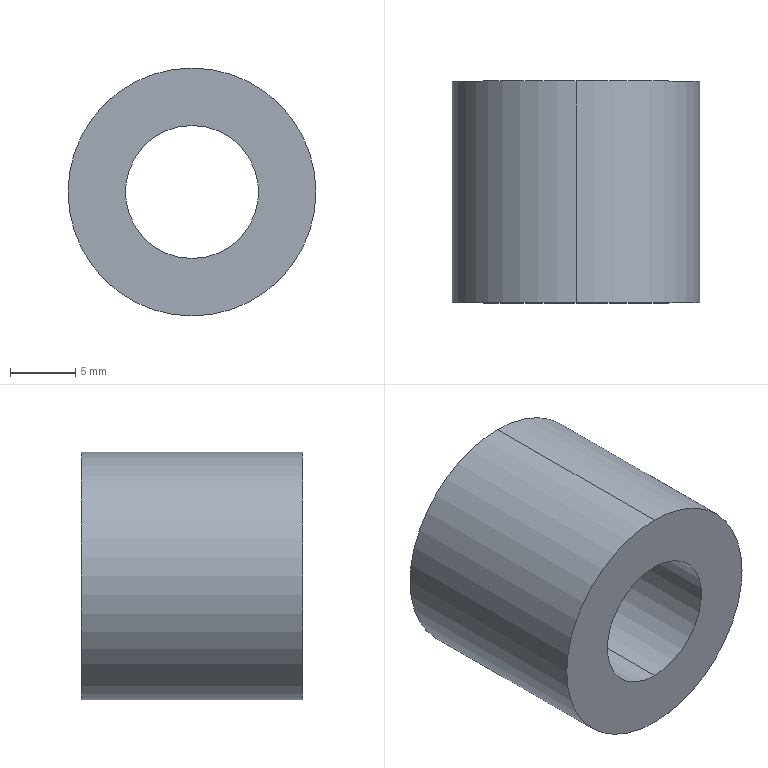Part | SolidWorks | features Extrusion 1, HoleWzd 1 | 1 solid | 6 faces | box 19 x 17 x 19 mm | volume 3431 mm3 | cylinder 4 | plane 2 | commonest cylinder face diameters 10.2 x2 19 x2
STEP:
#1=CARTESIAN_POINT('',(0.,0.,-5.1));
#2=VERTEX_POINT('',#1);
#3=CARTESIAN_POINT('',(0.,0.,5.1));
#4=VERTEX_POINT('',#3);
#5=CARTESIAN_POINT('',(0.,0.,0.));
#6=DIRECTION('',(0.,1.,0.));
#7=DIRECTION('',(0.,0.,1.));
#8=AXIS2_PLACEMENT_3D('',#5,#6,#7);
#9=CIRCLE('',#8,5.1);
#10=EDGE_CURVE('',#2,#4,#9,.T.);
#11=ORIENTED_EDGE('',*,*,#10,.F.);
#12=CARTESIAN_POINT('',(0.,17.,-5.1));
#13=VERTEX_POINT('',#12);
#14=CARTESIAN_POINT('',(0.,17.,-5.1));
#15=DIRECTION('',(0.,1.,0.));
#16=VECTOR('',#15,1000.);
#17=LINE('',#14,#16);
#18=EDGE_CURVE('',#2,#13,#17,.T.);
#19=ORIENTED_EDGE('',*,*,#18,.T.);
#20=CARTESIAN_POINT('',(0.,17.,5.1));
#21=VERTEX_POINT('',#20);
#22=CARTESIAN_POINT('',(0.,17.,0.));
#23=DIRECTION('',(0.,1.,0.));
#24=DIRECTION('',(0.,0.,1.));
#25=AXIS2_PLACEMENT_3D('',#22,#23,#24);
#26=CIRCLE('',#25,5.1);
#27=EDGE_CURVE('',#13,#21,#26,.T.);
#28=ORIENTED_EDGE('',*,*,#27,.T.);
#29=CARTESIAN_POINT('',(0.,17.,5.1));
#30=DIRECTION('',(0.,1.,0.));
#31=VECTOR('',#30,1000.);
#32=LINE('',#29,#31);
#33=EDGE_CURVE('',#4,#21,#32,.T.);
#34=ORIENTED_EDGE('',*,*,#33,.F.);
#35=EDGE_LOOP('',(#11,#19,#28,#34));
#36=FACE_OUTER_BOUND('',#35,.T.);
#37=CARTESIAN_POINT('',(0.,17.,0.));
#38=DIRECTION('',(0.,1.,0.));
#39=DIRECTION('',(0.,0.,1.));
#40=AXIS2_PLACEMENT_3D('',#37,#38,#39);
#41=CYLINDRICAL_SURFACE('',#40,5.1);
#42=ADVANCED_FACE('',(#36),#41,.F.);
#43=CARTESIAN_POINT('',(0.,17.,9.5));
#44=VERTEX_POINT('',#43);
#45=CARTESIAN_POINT('',(0.,17.,-9.5));
#46=VERTEX_POINT('',#45);
#47=CARTESIAN_POINT('',(0.,17.,0.));
#48=DIRECTION('',(0.,1.,0.));
#49=DIRECTION('',(0.,0.,1.));
#50=AXIS2_PLACEMENT_3D('',#47,#48,#49);
#51=CIRCLE('',#50,9.5);
#52=EDGE_CURVE('',#44,#46,#51,.T.);
#53=ORIENTED_EDGE('',*,*,#52,.F.);
#54=CARTESIAN_POINT('',(0.,0.,9.5));
#55=VERTEX_POINT('',#54);
#56=CARTESIAN_POINT('',(0.,17.,9.5));
#57=DIRECTION('',(0.,-1.,0.));
#58=VECTOR('',#57,1000.);
#59=LINE('',#56,#58);
#60=EDGE_CURVE('',#44,#55,#59,.T.);
#61=ORIENTED_EDGE('',*,*,#60,.T.);
#62=CARTESIAN_POINT('',(0.,0.,-9.5));
#63=VERTEX_POINT('',#62);
#64=CARTESIAN_POINT('',(0.,0.,0.));
#65=DIRECTION('',(0.,1.,0.));
#66=DIRECTION('',(0.,0.,1.));
#67=AXIS2_PLACEMENT_3D('',#64,#65,#66);
#68=CIRCLE('',#67,9.5);
#69=EDGE_CURVE('',#55,#63,#68,.T.);
#70=ORIENTED_EDGE('',*,*,#69,.T.);
#71=CARTESIAN_POINT('',(0.,17.,-9.5));
#72=DIRECTION('',(0.,-1.,0.));
#73=VECTOR('',#72,1000.);
#74=LINE('',#71,#73);
#75=EDGE_CURVE('',#46,#63,#74,.T.);
#76=ORIENTED_EDGE('',*,*,#75,.F.);
#77=EDGE_LOOP('',(#53,#61,#70,#76));
#78=FACE_OUTER_BOUND('',#77,.T.);
#79=CARTESIAN_POINT('',(0.,17.,0.));
#80=DIRECTION('',(0.,-1.,0.));
#81=DIRECTION('',(0.,0.,-1.));
#82=AXIS2_PLACEMENT_3D('',#79,#80,#81);
#83=CYLINDRICAL_SURFACE('',#82,9.5);
#84=ADVANCED_FACE('',(#78),#83,.T.);
#85=CARTESIAN_POINT('',(0.,17.,0.));
#86=DIRECTION('',(0.,1.,0.));
#87=DIRECTION('',(0.,0.,1.));
#88=AXIS2_PLACEMENT_3D('',#85,#86,#87);
#89=CIRCLE('',#88,5.1);
#90=EDGE_CURVE('',#21,#13,#89,.T.);
#91=ORIENTED_EDGE('',*,*,#90,.F.);
#92=ORIENTED_EDGE('',*,*,#27,.F.);
#93=EDGE_LOOP('',(#91,#92));
#94=FACE_BOUND('',#93,.T.);
#95=CARTESIAN_POINT('',(0.,17.,0.));
#96=DIRECTION('',(0.,1.,0.));
#97=DIRECTION('',(0.,0.,1.));
#98=AXIS2_PLACEMENT_3D('',#95,#96,#97);
#99=CIRCLE('',#98,9.5);
#100=EDGE_CURVE('',#46,#44,#99,.T.);
#101=ORIENTED_EDGE('',*,*,#100,.T.);
#102=ORIENTED_EDGE('',*,*,#52,.T.);
#103=EDGE_LOOP('',(#101,#102));
#104=FACE_OUTER_BOUND('',#103,.T.);
#105=CARTESIAN_POINT('',(0.,17.,0.));
#106=DIRECTION('',(0.,1.,0.));
#107=DIRECTION('',(0.,0.,1.));
#108=AXIS2_PLACEMENT_3D('',#105,#106,#107);
#109=PLANE('',#108);
#110=ADVANCED_FACE('',(#94,#104),#109,.T.);
#111=CARTESIAN_POINT('',(0.,0.,0.));
#112=DIRECTION('',(0.,1.,0.));
#113=DIRECTION('',(0.,0.,1.));
#114=AXIS2_PLACEMENT_3D('',#111,#112,#113);
#115=CIRCLE('',#114,5.1);
#116=EDGE_CURVE('',#4,#2,#115,.T.);
#117=ORIENTED_EDGE('',*,*,#116,.T.);
#118=ORIENTED_EDGE('',*,*,#10,.T.);
#119=EDGE_LOOP('',(#117,#118));
#120=FACE_BOUND('',#119,.T.);
#121=CARTESIAN_POINT('',(0.,0.,0.));
#122=DIRECTION('',(0.,1.,0.));
#123=DIRECTION('',(0.,0.,1.));
#124=AXIS2_PLACEMENT_3D('',#121,#122,#123);
#125=CIRCLE('',#124,9.5);
#126=EDGE_CURVE('',#63,#55,#125,.T.);
#127=ORIENTED_EDGE('',*,*,#126,.F.);
#128=ORIENTED_EDGE('',*,*,#69,.F.);
#129=EDGE_LOOP('',(#127,#128));
#130=FACE_OUTER_BOUND('',#129,.T.);
#131=CARTESIAN_POINT('',(0.,0.,0.));
#132=DIRECTION('',(0.,1.,0.));
#133=DIRECTION('',(0.,0.,1.));
#134=AXIS2_PLACEMENT_3D('',#131,#132,#133);
#135=PLANE('',#134);
#136=ADVANCED_FACE('',(#120,#130),#135,.F.);
#137=ORIENTED_EDGE('',*,*,#60,.F.);
#138=ORIENTED_EDGE('',*,*,#100,.F.);
#139=ORIENTED_EDGE('',*,*,#75,.T.);
#140=ORIENTED_EDGE('',*,*,#126,.T.);
#141=EDGE_LOOP('',(#137,#138,#139,#140));
#142=FACE_OUTER_BOUND('',#141,.T.);
#143=CARTESIAN_POINT('',(0.,17.,0.));
#144=DIRECTION('',(0.,-1.,0.));
#145=DIRECTION('',(0.,0.,-1.));
#146=AXIS2_PLACEMENT_3D('',#143,#144,#145);
#147=CYLINDRICAL_SURFACE('',#146,9.5);
#148=ADVANCED_FACE('',(#142),#147,.T.);
#149=ORIENTED_EDGE('',*,*,#18,.F.);
#150=ORIENTED_EDGE('',*,*,#116,.F.);
#151=ORIENTED_EDGE('',*,*,#33,.T.);
#152=ORIENTED_EDGE('',*,*,#90,.T.);
#153=EDGE_LOOP('',(#149,#150,#151,#152));
#154=FACE_OUTER_BOUND('',#153,.T.);
#155=CARTESIAN_POINT('',(0.,17.,0.));
#156=DIRECTION('',(0.,1.,0.));
#157=DIRECTION('',(0.,0.,1.));
#158=AXIS2_PLACEMENT_3D('',#155,#156,#157);
#159=CYLINDRICAL_SURFACE('',#158,5.1);
#160=ADVANCED_FACE('',(#154),#159,.F.);
#161=CLOSED_SHELL('',(#42,#84,#110,#136,#148,#160));
#162=MANIFOLD_SOLID_BREP('',#161);
#163=CARTESIAN_POINT('',(0.,0.,0.));
#164=DIRECTION('',(0.,0.,1.));
#165=DIRECTION('',(1.,0.,0.));
#166=AXIS2_PLACEMENT_3D('',#163,#164,#165);
#167=(LENGTH_UNIT()NAMED_UNIT(*)SI_UNIT(.MILLI.,.METRE.));
#168=UNCERTAINTY_MEASURE_WITH_UNIT(LENGTH_MEASURE(0.00001),#167,'','');
#169=(NAMED_UNIT(*)PLANE_ANGLE_UNIT()SI_UNIT($,.RADIAN.));
#170=(NAMED_UNIT(*)SI_UNIT($,.STERADIAN.)SOLID_ANGLE_UNIT());
#171=(GEOMETRIC_REPRESENTATION_CONTEXT(3)GLOBAL_UNCERTAINTY_ASSIGNED_CONTEXT((#168))GLOBAL_UNIT_ASSIGNED_CONTEXT((#167,#169,#170))REPRESENTATION_CONTEXT('',''));
#172=ADVANCED_BREP_SHAPE_REPRESENTATION('',(#162,#166),#171);